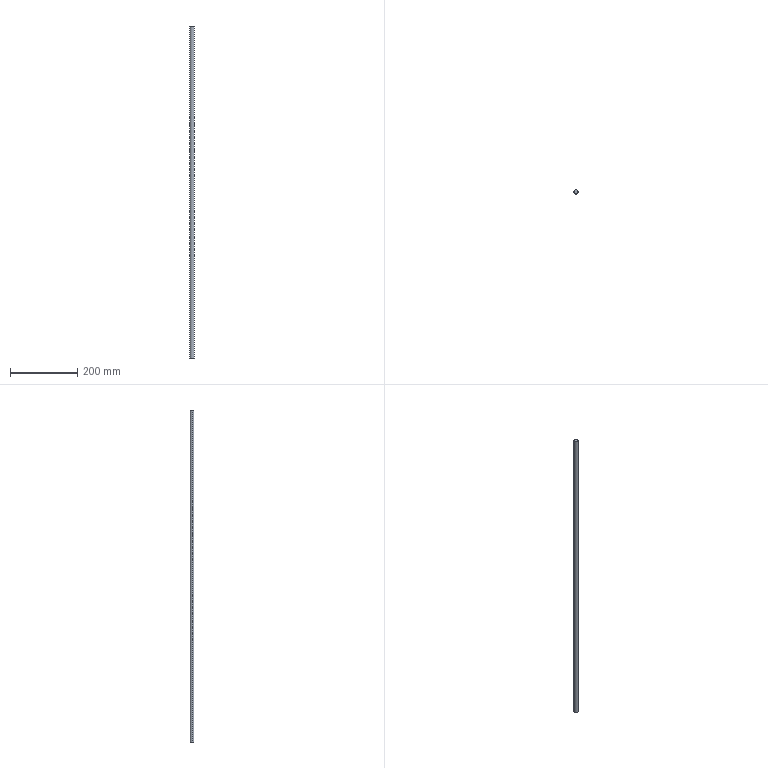Part | SolidWorks | features BaseBody 1 | 1 solid | 4 faces | box 12 x 12 x 990 mm | volume 111966 mm3 | cylinder 2 | plane 2 | commonest cylinder face diameters 12 x2
STEP:
#1=CARTESIAN_POINT('',(-6.,0.,990.));
#2=VERTEX_POINT('',#1);
#3=CARTESIAN_POINT('',(6.,0.,990.));
#4=VERTEX_POINT('',#3);
#5=CARTESIAN_POINT('',(0.,0.,990.));
#6=DIRECTION('',(0.,0.,-1.));
#7=DIRECTION('',(-1.,0.,0.));
#8=AXIS2_PLACEMENT_3D('',#5,#6,#7);
#9=CIRCLE('',#8,6.);
#10=EDGE_CURVE('',#2,#4,#9,.T.);
#11=ORIENTED_EDGE('',*,*,#10,.T.);
#12=CARTESIAN_POINT('',(6.,0.,0.));
#13=VERTEX_POINT('',#12);
#14=CARTESIAN_POINT('',(6.,0.,990.));
#15=DIRECTION('',(0.,0.,-1.));
#16=VECTOR('',#15,1000.);
#17=LINE('',#14,#16);
#18=EDGE_CURVE('',#4,#13,#17,.T.);
#19=ORIENTED_EDGE('',*,*,#18,.T.);
#20=CARTESIAN_POINT('',(-6.,0.,0.));
#21=VERTEX_POINT('',#20);
#22=CARTESIAN_POINT('',(0.,0.,0.));
#23=DIRECTION('',(0.,0.,1.));
#24=DIRECTION('',(-1.,0.,0.));
#25=AXIS2_PLACEMENT_3D('',#22,#23,#24);
#26=CIRCLE('',#25,6.);
#27=EDGE_CURVE('',#13,#21,#26,.T.);
#28=ORIENTED_EDGE('',*,*,#27,.T.);
#29=CARTESIAN_POINT('',(-6.,0.,990.));
#30=DIRECTION('',(0.,0.,-1.));
#31=VECTOR('',#30,1000.);
#32=LINE('',#29,#31);
#33=EDGE_CURVE('',#2,#21,#32,.T.);
#34=ORIENTED_EDGE('',*,*,#33,.F.);
#35=EDGE_LOOP('',(#11,#19,#28,#34));
#36=FACE_OUTER_BOUND('',#35,.T.);
#37=CARTESIAN_POINT('',(0.,0.,990.));
#38=DIRECTION('',(0.,0.,-1.));
#39=DIRECTION('',(-1.,0.,0.));
#40=AXIS2_PLACEMENT_3D('',#37,#38,#39);
#41=CYLINDRICAL_SURFACE('',#40,6.);
#42=ADVANCED_FACE('',(#36),#41,.T.);
#43=ORIENTED_EDGE('',*,*,#18,.F.);
#44=CARTESIAN_POINT('',(0.,0.,990.));
#45=DIRECTION('',(0.,0.,-1.));
#46=DIRECTION('',(-1.,0.,0.));
#47=AXIS2_PLACEMENT_3D('',#44,#45,#46);
#48=CIRCLE('',#47,6.);
#49=EDGE_CURVE('',#4,#2,#48,.T.);
#50=ORIENTED_EDGE('',*,*,#49,.T.);
#51=ORIENTED_EDGE('',*,*,#33,.T.);
#52=CARTESIAN_POINT('',(0.,0.,0.));
#53=DIRECTION('',(0.,0.,1.));
#54=DIRECTION('',(-1.,0.,0.));
#55=AXIS2_PLACEMENT_3D('',#52,#53,#54);
#56=CIRCLE('',#55,6.);
#57=EDGE_CURVE('',#21,#13,#56,.T.);
#58=ORIENTED_EDGE('',*,*,#57,.T.);
#59=EDGE_LOOP('',(#43,#50,#51,#58));
#60=FACE_OUTER_BOUND('',#59,.T.);
#61=CARTESIAN_POINT('',(0.,0.,990.));
#62=DIRECTION('',(0.,0.,-1.));
#63=DIRECTION('',(-1.,0.,0.));
#64=AXIS2_PLACEMENT_3D('',#61,#62,#63);
#65=CYLINDRICAL_SURFACE('',#64,6.);
#66=ADVANCED_FACE('',(#60),#65,.T.);
#67=ORIENTED_EDGE('',*,*,#57,.F.);
#68=ORIENTED_EDGE('',*,*,#27,.F.);
#69=EDGE_LOOP('',(#67,#68));
#70=FACE_OUTER_BOUND('',#69,.T.);
#71=CARTESIAN_POINT('',(0.,0.,0.));
#72=DIRECTION('',(0.,0.,1.));
#73=DIRECTION('',(1.,0.,0.));
#74=AXIS2_PLACEMENT_3D('',#71,#72,#73);
#75=PLANE('',#74);
#76=ADVANCED_FACE('',(#70),#75,.F.);
#77=ORIENTED_EDGE('',*,*,#10,.F.);
#78=ORIENTED_EDGE('',*,*,#49,.F.);
#79=EDGE_LOOP('',(#77,#78));
#80=FACE_OUTER_BOUND('',#79,.T.);
#81=CARTESIAN_POINT('',(0.,0.,990.));
#82=DIRECTION('',(0.,0.,1.));
#83=DIRECTION('',(1.,0.,0.));
#84=AXIS2_PLACEMENT_3D('',#81,#82,#83);
#85=PLANE('',#84);
#86=ADVANCED_FACE('',(#80),#85,.T.);
#87=CLOSED_SHELL('',(#42,#66,#76,#86));
#88=MANIFOLD_SOLID_BREP('',#87);
#89=CARTESIAN_POINT('',(0.,0.,0.));
#90=DIRECTION('',(0.,0.,1.));
#91=DIRECTION('',(1.,0.,0.));
#92=AXIS2_PLACEMENT_3D('',#89,#90,#91);
#93=(LENGTH_UNIT()NAMED_UNIT(*)SI_UNIT(.MILLI.,.METRE.));
#94=UNCERTAINTY_MEASURE_WITH_UNIT(LENGTH_MEASURE(0.00001),#93,'','');
#95=(NAMED_UNIT(*)PLANE_ANGLE_UNIT()SI_UNIT($,.RADIAN.));
#96=(NAMED_UNIT(*)SI_UNIT($,.STERADIAN.)SOLID_ANGLE_UNIT());
#97=(GEOMETRIC_REPRESENTATION_CONTEXT(3)GLOBAL_UNCERTAINTY_ASSIGNED_CONTEXT((#94))GLOBAL_UNIT_ASSIGNED_CONTEXT((#93,#95,#96))REPRESENTATION_CONTEXT('',''));
#98=ADVANCED_BREP_SHAPE_REPRESENTATION('',(#88,#92),#97);